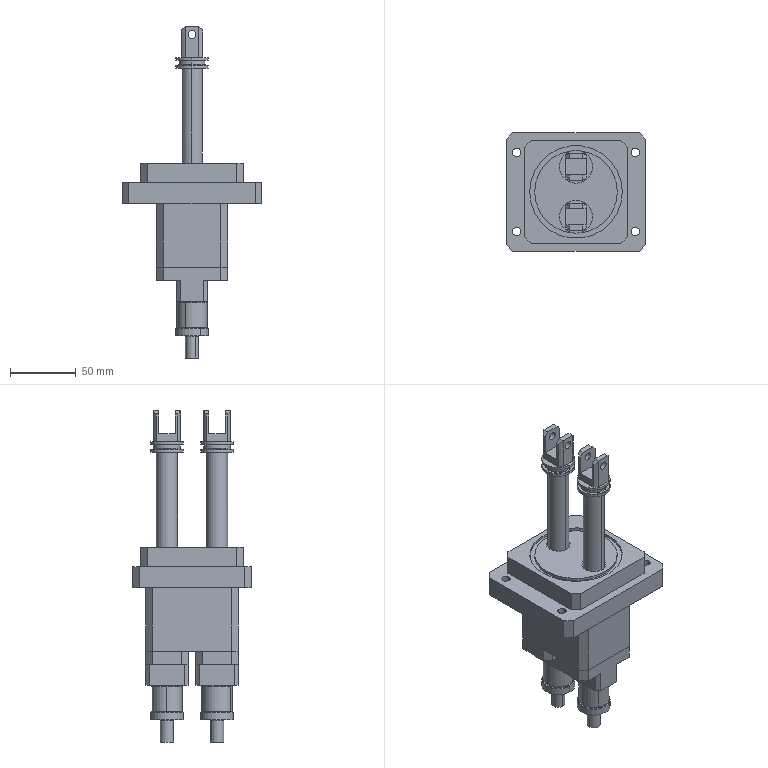Part | SolidWorks | 9 solids | 378 faces | box 106 x 90 x 252 mm | volume 513009 mm3 | plane 142 | cylinder 140 | cone 64 | torus 32 | commonest cylinder face diameters 10 x16 16 x12 23 x12 25 x12 4.2 x8 5 x8